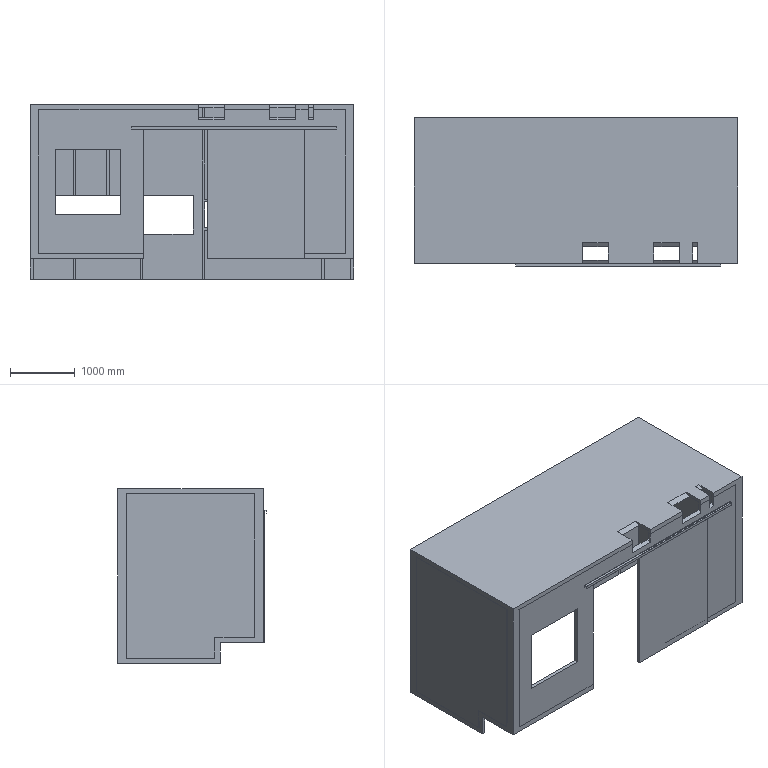Part | NX | features BREP 2 | 2 solids | 158 faces | box 5000 x 2295 x 2700 mm | volume 2137784674 mm3 | plane 158